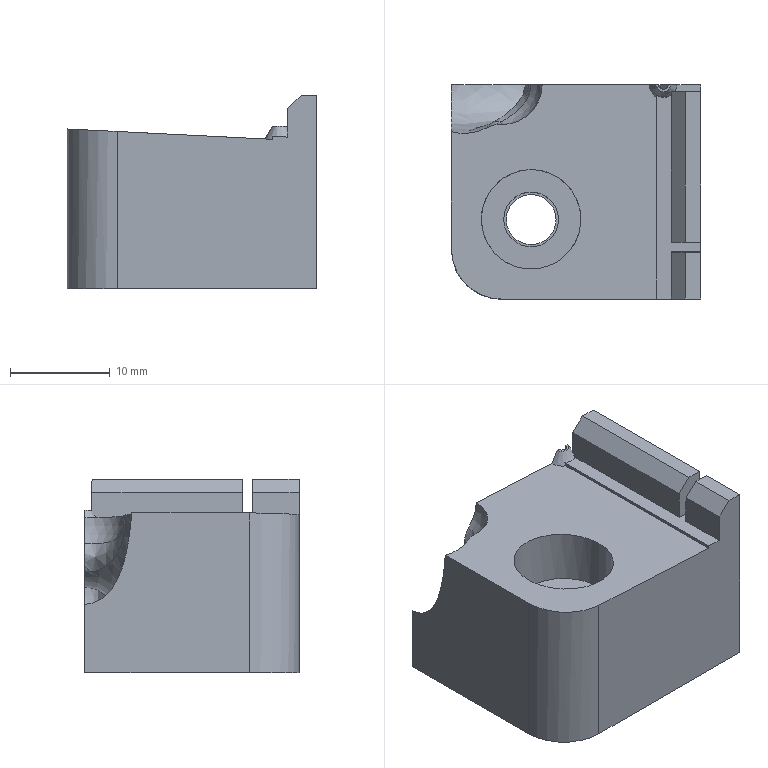Part | STEP file | solid 200 | 1 solid | 36 faces | box 25 x 21.516 x 19.435 mm | volume 7252 mm3 | plane 17 | spline 10 | cylinder 7 | sphere 1 | cone 1 | commonest cylinder face diameters 10 x2 6922 x2 5 x1 5.5 x1 8 x1